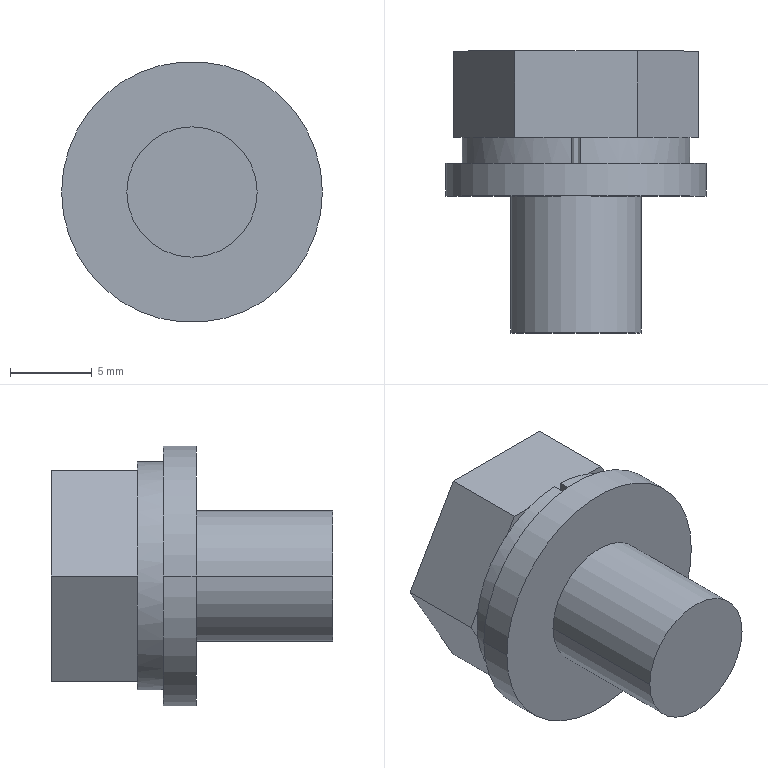Part | STEP file | LIB_36623144_M8X12 | 1 solid | 32 faces | box 16 x 17.3 x 16 mm | volume 1844 mm3 | plane 26 | cylinder 6 | commonest cylinder face diameters 8 x3 16 x2 14 x1